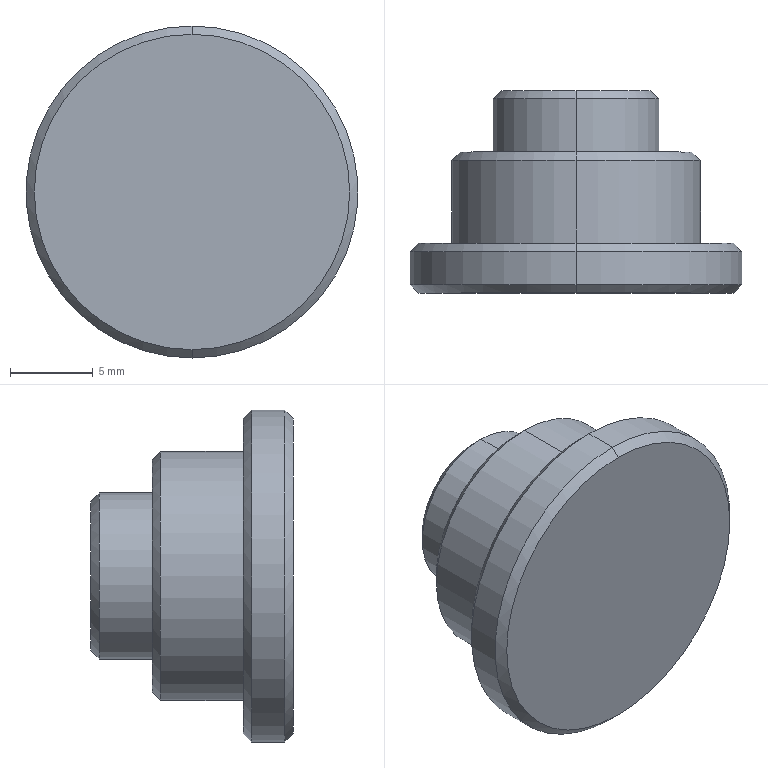Part | SolidWorks | features Chamfer 1, Revolution 1 | 1 solid | 18 faces | box 20 x 12.2 x 20 mm | volume 2180 mm3 | cone 8 | cylinder 6 | plane 4 | commonest cylinder face diameters 10 x2 15 x2 20 x2
STEP:
#1=CARTESIAN_POINT('',(136.663,-334.304,4.5));
#2=VERTEX_POINT('',#1);
#3=CARTESIAN_POINT('',(136.663,-334.304,-4.5));
#4=VERTEX_POINT('',#3);
#5=CARTESIAN_POINT('',(136.663,-334.304,0.));
#6=DIRECTION('',(0.,1.,0.));
#7=DIRECTION('',(0.,0.,-1.));
#8=AXIS2_PLACEMENT_3D('',#5,#6,#7);
#9=CIRCLE('',#8,4.5);
#10=EDGE_CURVE('',#2,#4,#9,.T.);
#11=ORIENTED_EDGE('',*,*,#10,.F.);
#12=CARTESIAN_POINT('',(136.663,-334.804,5.));
#13=VERTEX_POINT('',#12);
#14=CARTESIAN_POINT('',(136.663,-334.804,5.));
#15=DIRECTION('',(0.,-0.7071,0.7071));
#16=VECTOR('',#15,1000.);
#17=LINE('',#14,#16);
#18=EDGE_CURVE('',#2,#13,#17,.T.);
#19=ORIENTED_EDGE('',*,*,#18,.T.);
#20=CARTESIAN_POINT('',(136.663,-334.804,-5.));
#21=VERTEX_POINT('',#20);
#22=CARTESIAN_POINT('',(136.663,-334.804,0.));
#23=DIRECTION('',(0.,-1.,0.));
#24=DIRECTION('',(0.,0.,-1.));
#25=AXIS2_PLACEMENT_3D('',#22,#23,#24);
#26=CIRCLE('',#25,5.);
#27=EDGE_CURVE('',#21,#13,#26,.T.);
#28=ORIENTED_EDGE('',*,*,#27,.F.);
#29=CARTESIAN_POINT('',(136.663,-334.804,-5.));
#30=DIRECTION('',(0.,-0.7071,-0.7071));
#31=VECTOR('',#30,1000.);
#32=LINE('',#29,#31);
#33=EDGE_CURVE('',#4,#21,#32,.T.);
#34=ORIENTED_EDGE('',*,*,#33,.F.);
#35=EDGE_LOOP('',(#11,#19,#28,#34));
#36=FACE_OUTER_BOUND('',#35,.T.);
#37=CARTESIAN_POINT('',(136.663,-334.804,0.));
#38=DIRECTION('',(0.,-1.,0.));
#39=DIRECTION('',(0.,0.,-1.));
#40=AXIS2_PLACEMENT_3D('',#37,#38,#39);
#41=CONICAL_SURFACE('',#40,5.,0.7854);
#42=ADVANCED_FACE('',(#36),#41,.T.);
#43=CARTESIAN_POINT('',(136.663,-338.004,7.));
#44=VERTEX_POINT('',#43);
#45=CARTESIAN_POINT('',(136.663,-338.004,-7.));
#46=VERTEX_POINT('',#45);
#47=CARTESIAN_POINT('',(136.663,-338.004,0.));
#48=DIRECTION('',(0.,1.,0.));
#49=DIRECTION('',(0.,0.,-1.));
#50=AXIS2_PLACEMENT_3D('',#47,#48,#49);
#51=CIRCLE('',#50,7.);
#52=EDGE_CURVE('',#44,#46,#51,.T.);
#53=ORIENTED_EDGE('',*,*,#52,.F.);
#54=CARTESIAN_POINT('',(136.663,-338.504,7.5));
#55=VERTEX_POINT('',#54);
#56=CARTESIAN_POINT('',(136.663,-338.504,7.5));
#57=DIRECTION('',(0.,-0.7071,0.7071));
#58=VECTOR('',#57,1000.);
#59=LINE('',#56,#58);
#60=EDGE_CURVE('',#44,#55,#59,.T.);
#61=ORIENTED_EDGE('',*,*,#60,.T.);
#62=CARTESIAN_POINT('',(136.663,-338.504,-7.5));
#63=VERTEX_POINT('',#62);
#64=CARTESIAN_POINT('',(136.663,-338.504,0.));
#65=DIRECTION('',(0.,-1.,0.));
#66=DIRECTION('',(0.,0.,-1.));
#67=AXIS2_PLACEMENT_3D('',#64,#65,#66);
#68=CIRCLE('',#67,7.5);
#69=EDGE_CURVE('',#63,#55,#68,.T.);
#70=ORIENTED_EDGE('',*,*,#69,.F.);
#71=CARTESIAN_POINT('',(136.663,-338.504,-7.5));
#72=DIRECTION('',(0.,-0.7071,-0.7071));
#73=VECTOR('',#72,1000.);
#74=LINE('',#71,#73);
#75=EDGE_CURVE('',#46,#63,#74,.T.);
#76=ORIENTED_EDGE('',*,*,#75,.F.);
#77=EDGE_LOOP('',(#53,#61,#70,#76));
#78=FACE_OUTER_BOUND('',#77,.T.);
#79=CARTESIAN_POINT('',(136.663,-338.504,0.));
#80=DIRECTION('',(0.,-1.,0.));
#81=DIRECTION('',(0.,0.,-1.));
#82=AXIS2_PLACEMENT_3D('',#79,#80,#81);
#83=CONICAL_SURFACE('',#82,7.5,0.7854);
#84=ADVANCED_FACE('',(#78),#83,.T.);
#85=CARTESIAN_POINT('',(136.663,-343.504,9.5));
#86=VERTEX_POINT('',#85);
#87=CARTESIAN_POINT('',(136.663,-343.504,-9.5));
#88=VERTEX_POINT('',#87);
#89=CARTESIAN_POINT('',(136.663,-343.504,0.));
#90=DIRECTION('',(0.,1.,0.));
#91=DIRECTION('',(0.,0.,-1.));
#92=AXIS2_PLACEMENT_3D('',#89,#90,#91);
#93=CIRCLE('',#92,9.5);
#94=EDGE_CURVE('',#86,#88,#93,.T.);
#95=ORIENTED_EDGE('',*,*,#94,.F.);
#96=CARTESIAN_POINT('',(136.663,-344.004,10.));
#97=VERTEX_POINT('',#96);
#98=CARTESIAN_POINT('',(136.663,-344.004,10.));
#99=DIRECTION('',(0.,-0.7071,0.7071));
#100=VECTOR('',#99,1000.);
#101=LINE('',#98,#100);
#102=EDGE_CURVE('',#86,#97,#101,.T.);
#103=ORIENTED_EDGE('',*,*,#102,.T.);
#104=CARTESIAN_POINT('',(136.663,-344.004,-10.));
#105=VERTEX_POINT('',#104);
#106=CARTESIAN_POINT('',(136.663,-344.004,0.));
#107=DIRECTION('',(0.,-1.,0.));
#108=DIRECTION('',(0.,0.,-1.));
#109=AXIS2_PLACEMENT_3D('',#106,#107,#108);
#110=CIRCLE('',#109,10.);
#111=EDGE_CURVE('',#105,#97,#110,.T.);
#112=ORIENTED_EDGE('',*,*,#111,.F.);
#113=CARTESIAN_POINT('',(136.663,-344.004,-10.));
#114=DIRECTION('',(0.,-0.7071,-0.7071));
#115=VECTOR('',#114,1000.);
#116=LINE('',#113,#115);
#117=EDGE_CURVE('',#88,#105,#116,.T.);
#118=ORIENTED_EDGE('',*,*,#117,.F.);
#119=EDGE_LOOP('',(#95,#103,#112,#118));
#120=FACE_OUTER_BOUND('',#119,.T.);
#121=CARTESIAN_POINT('',(136.663,-344.004,0.));
#122=DIRECTION('',(0.,-1.,0.));
#123=DIRECTION('',(0.,0.,-1.));
#124=AXIS2_PLACEMENT_3D('',#121,#122,#123);
#125=CONICAL_SURFACE('',#124,10.,0.7854);
#126=ADVANCED_FACE('',(#120),#125,.T.);
#127=CARTESIAN_POINT('',(136.663,-346.504,-9.5));
#128=VERTEX_POINT('',#127);
#129=CARTESIAN_POINT('',(136.663,-346.504,9.5));
#130=VERTEX_POINT('',#129);
#131=CARTESIAN_POINT('',(136.663,-346.504,0.));
#132=DIRECTION('',(0.,-1.,0.));
#133=DIRECTION('',(0.,0.,1.));
#134=AXIS2_PLACEMENT_3D('',#131,#132,#133);
#135=CIRCLE('',#134,9.5);
#136=EDGE_CURVE('',#128,#130,#135,.T.);
#137=ORIENTED_EDGE('',*,*,#136,.F.);
#138=CARTESIAN_POINT('',(136.663,-346.004,-10.));
#139=VERTEX_POINT('',#138);
#140=CARTESIAN_POINT('',(136.663,-346.504,-9.5));
#141=DIRECTION('',(0.,0.7071,-0.7071));
#142=VECTOR('',#141,1000.);
#143=LINE('',#140,#142);
#144=EDGE_CURVE('',#128,#139,#143,.T.);
#145=ORIENTED_EDGE('',*,*,#144,.T.);
#146=CARTESIAN_POINT('',(136.663,-346.004,10.));
#147=VERTEX_POINT('',#146);
#148=CARTESIAN_POINT('',(136.663,-346.004,0.));
#149=DIRECTION('',(0.,1.,0.));
#150=DIRECTION('',(0.,0.,1.));
#151=AXIS2_PLACEMENT_3D('',#148,#149,#150);
#152=CIRCLE('',#151,10.);
#153=EDGE_CURVE('',#147,#139,#152,.T.);
#154=ORIENTED_EDGE('',*,*,#153,.F.);
#155=CARTESIAN_POINT('',(136.663,-346.504,9.5));
#156=DIRECTION('',(0.,0.7071,0.7071));
#157=VECTOR('',#156,1000.);
#158=LINE('',#155,#157);
#159=EDGE_CURVE('',#130,#147,#158,.T.);
#160=ORIENTED_EDGE('',*,*,#159,.F.);
#161=EDGE_LOOP('',(#137,#145,#154,#160));
#162=FACE_OUTER_BOUND('',#161,.T.);
#163=CARTESIAN_POINT('',(136.663,-346.504,0.));
#164=DIRECTION('',(0.,1.,0.));
#165=DIRECTION('',(0.,0.,1.));
#166=AXIS2_PLACEMENT_3D('',#163,#164,#165);
#167=CONICAL_SURFACE('',#166,9.5,0.7854);
#168=ADVANCED_FACE('',(#162),#167,.T.);
#169=ORIENTED_EDGE('',*,*,#111,.T.);
#170=CARTESIAN_POINT('',(136.663,-346.504,10.));
#171=DIRECTION('',(0.,-1.,0.));
#172=VECTOR('',#171,1000.);
#173=LINE('',#170,#172);
#174=EDGE_CURVE('',#97,#147,#173,.T.);
#175=ORIENTED_EDGE('',*,*,#174,.T.);
#176=ORIENTED_EDGE('',*,*,#153,.T.);
#177=CARTESIAN_POINT('',(136.663,-346.504,-10.));
#178=DIRECTION('',(0.,-1.,0.));
#179=VECTOR('',#178,1000.);
#180=LINE('',#177,#179);
#181=EDGE_CURVE('',#105,#139,#180,.T.);
#182=ORIENTED_EDGE('',*,*,#181,.F.);
#183=EDGE_LOOP('',(#169,#175,#176,#182));
#184=FACE_OUTER_BOUND('',#183,.T.);
#185=CARTESIAN_POINT('',(136.663,-346.504,0.));
#186=DIRECTION('',(0.,-1.,0.));
#187=DIRECTION('',(0.,0.,-1.));
#188=AXIS2_PLACEMENT_3D('',#185,#186,#187);
#189=CYLINDRICAL_SURFACE('',#188,10.);
#190=ADVANCED_FACE('',(#184),#189,.T.);
#191=ORIENTED_EDGE('',*,*,#69,.T.);
#192=CARTESIAN_POINT('',(136.663,-343.504,7.5));
#193=VERTEX_POINT('',#192);
#194=CARTESIAN_POINT('',(136.663,-346.504,7.5));
#195=DIRECTION('',(0.,-1.,0.));
#196=VECTOR('',#195,1000.);
#197=LINE('',#194,#196);
#198=EDGE_CURVE('',#55,#193,#197,.T.);
#199=ORIENTED_EDGE('',*,*,#198,.T.);
#200=CARTESIAN_POINT('',(136.663,-343.504,-7.5));
#201=VERTEX_POINT('',#200);
#202=CARTESIAN_POINT('',(136.663,-343.504,0.));
#203=DIRECTION('',(0.,-1.,0.));
#204=DIRECTION('',(0.,0.,-1.));
#205=AXIS2_PLACEMENT_3D('',#202,#203,#204);
#206=CIRCLE('',#205,7.5);
#207=EDGE_CURVE('',#201,#193,#206,.T.);
#208=ORIENTED_EDGE('',*,*,#207,.F.);
#209=CARTESIAN_POINT('',(136.663,-346.504,-7.5));
#210=DIRECTION('',(0.,-1.,0.));
#211=VECTOR('',#210,1000.);
#212=LINE('',#209,#211);
#213=EDGE_CURVE('',#63,#201,#212,.T.);
#214=ORIENTED_EDGE('',*,*,#213,.F.);
#215=EDGE_LOOP('',(#191,#199,#208,#214));
#216=FACE_OUTER_BOUND('',#215,.T.);
#217=CARTESIAN_POINT('',(136.663,-346.504,0.));
#218=DIRECTION('',(0.,-1.,0.));
#219=DIRECTION('',(0.,0.,-1.));
#220=AXIS2_PLACEMENT_3D('',#217,#218,#219);
#221=CYLINDRICAL_SURFACE('',#220,7.5);
#222=ADVANCED_FACE('',(#216),#221,.T.);
#223=ORIENTED_EDGE('',*,*,#27,.T.);
#224=CARTESIAN_POINT('',(136.663,-338.004,5.));
#225=VERTEX_POINT('',#224);
#226=CARTESIAN_POINT('',(136.663,-346.504,5.));
#227=DIRECTION('',(0.,-1.,0.));
#228=VECTOR('',#227,1000.);
#229=LINE('',#226,#228);
#230=EDGE_CURVE('',#13,#225,#229,.T.);
#231=ORIENTED_EDGE('',*,*,#230,.T.);
#232=CARTESIAN_POINT('',(136.663,-338.004,-5.));
#233=VERTEX_POINT('',#232);
#234=CARTESIAN_POINT('',(136.663,-338.004,0.));
#235=DIRECTION('',(0.,-1.,0.));
#236=DIRECTION('',(0.,0.,-1.));
#237=AXIS2_PLACEMENT_3D('',#234,#235,#236);
#238=CIRCLE('',#237,5.);
#239=EDGE_CURVE('',#233,#225,#238,.T.);
#240=ORIENTED_EDGE('',*,*,#239,.F.);
#241=CARTESIAN_POINT('',(136.663,-346.504,-5.));
#242=DIRECTION('',(0.,-1.,0.));
#243=VECTOR('',#242,1000.);
#244=LINE('',#241,#243);
#245=EDGE_CURVE('',#21,#233,#244,.T.);
#246=ORIENTED_EDGE('',*,*,#245,.F.);
#247=EDGE_LOOP('',(#223,#231,#240,#246));
#248=FACE_OUTER_BOUND('',#247,.T.);
#249=CARTESIAN_POINT('',(136.663,-346.504,0.));
#250=DIRECTION('',(0.,-1.,0.));
#251=DIRECTION('',(0.,0.,-1.));
#252=AXIS2_PLACEMENT_3D('',#249,#250,#251);
#253=CYLINDRICAL_SURFACE('',#252,5.);
#254=ADVANCED_FACE('',(#248),#253,.T.);
#255=CARTESIAN_POINT('',(136.663,-334.304,0.));
#256=DIRECTION('',(0.,1.,0.));
#257=DIRECTION('',(0.,0.,-1.));
#258=AXIS2_PLACEMENT_3D('',#255,#256,#257);
#259=CIRCLE('',#258,4.5);
#260=EDGE_CURVE('',#4,#2,#259,.T.);
#261=ORIENTED_EDGE('',*,*,#260,.T.);
#262=ORIENTED_EDGE('',*,*,#10,.T.);
#263=EDGE_LOOP('',(#261,#262));
#264=FACE_OUTER_BOUND('',#263,.T.);
#265=CARTESIAN_POINT('',(136.663,-334.304,0.));
#266=DIRECTION('',(0.,-1.,0.));
#267=DIRECTION('',(0.,0.,-1.));
#268=AXIS2_PLACEMENT_3D('',#265,#266,#267);
#269=PLANE('',#268);
#270=ADVANCED_FACE('',(#264),#269,.F.);
#271=ORIENTED_EDGE('',*,*,#230,.F.);
#272=CARTESIAN_POINT('',(136.663,-334.804,0.));
#273=DIRECTION('',(0.,-1.,0.));
#274=DIRECTION('',(0.,0.,-1.));
#275=AXIS2_PLACEMENT_3D('',#272,#273,#274);
#276=CIRCLE('',#275,5.);
#277=EDGE_CURVE('',#13,#21,#276,.T.);
#278=ORIENTED_EDGE('',*,*,#277,.T.);
#279=ORIENTED_EDGE('',*,*,#245,.T.);
#280=CARTESIAN_POINT('',(136.663,-338.004,0.));
#281=DIRECTION('',(0.,-1.,0.));
#282=DIRECTION('',(0.,0.,-1.));
#283=AXIS2_PLACEMENT_3D('',#280,#281,#282);
#284=CIRCLE('',#283,5.);
#285=EDGE_CURVE('',#225,#233,#284,.T.);
#286=ORIENTED_EDGE('',*,*,#285,.F.);
#287=EDGE_LOOP('',(#271,#278,#279,#286));
#288=FACE_OUTER_BOUND('',#287,.T.);
#289=CARTESIAN_POINT('',(136.663,-346.504,0.));
#290=DIRECTION('',(0.,-1.,0.));
#291=DIRECTION('',(0.,0.,-1.));
#292=AXIS2_PLACEMENT_3D('',#289,#290,#291);
#293=CYLINDRICAL_SURFACE('',#292,5.);
#294=ADVANCED_FACE('',(#288),#293,.T.);
#295=CARTESIAN_POINT('',(136.663,-338.004,0.));
#296=DIRECTION('',(0.,1.,0.));
#297=DIRECTION('',(0.,0.,-1.));
#298=AXIS2_PLACEMENT_3D('',#295,#296,#297);
#299=CIRCLE('',#298,7.);
#300=EDGE_CURVE('',#46,#44,#299,.T.);
#301=ORIENTED_EDGE('',*,*,#300,.T.);
#302=ORIENTED_EDGE('',*,*,#52,.T.);
#303=EDGE_LOOP('',(#301,#302));
#304=FACE_OUTER_BOUND('',#303,.T.);
#305=ORIENTED_EDGE('',*,*,#239,.T.);
#306=ORIENTED_EDGE('',*,*,#285,.T.);
#307=EDGE_LOOP('',(#305,#306));
#308=FACE_BOUND('',#307,.T.);
#309=CARTESIAN_POINT('',(131.663,-338.004,0.));
#310=DIRECTION('',(0.,-1.,0.));
#311=DIRECTION('',(0.,0.,-1.));
#312=AXIS2_PLACEMENT_3D('',#309,#310,#311);
#313=PLANE('',#312);
#314=ADVANCED_FACE('',(#304,#308),#313,.F.);
#315=ORIENTED_EDGE('',*,*,#198,.F.);
#316=CARTESIAN_POINT('',(136.663,-338.504,0.));
#317=DIRECTION('',(0.,-1.,0.));
#318=DIRECTION('',(0.,0.,-1.));
#319=AXIS2_PLACEMENT_3D('',#316,#317,#318);
#320=CIRCLE('',#319,7.5);
#321=EDGE_CURVE('',#55,#63,#320,.T.);
#322=ORIENTED_EDGE('',*,*,#321,.T.);
#323=ORIENTED_EDGE('',*,*,#213,.T.);
#324=CARTESIAN_POINT('',(136.663,-343.504,0.));
#325=DIRECTION('',(0.,-1.,0.));
#326=DIRECTION('',(0.,0.,-1.));
#327=AXIS2_PLACEMENT_3D('',#324,#325,#326);
#328=CIRCLE('',#327,7.5);
#329=EDGE_CURVE('',#193,#201,#328,.T.);
#330=ORIENTED_EDGE('',*,*,#329,.F.);
#331=EDGE_LOOP('',(#315,#322,#323,#330));
#332=FACE_OUTER_BOUND('',#331,.T.);
#333=CARTESIAN_POINT('',(136.663,-346.504,0.));
#334=DIRECTION('',(0.,-1.,0.));
#335=DIRECTION('',(0.,0.,-1.));
#336=AXIS2_PLACEMENT_3D('',#333,#334,#335);
#337=CYLINDRICAL_SURFACE('',#336,7.5);
#338=ADVANCED_FACE('',(#332),#337,.T.);
#339=CARTESIAN_POINT('',(136.663,-343.504,0.));
#340=DIRECTION('',(0.,1.,0.));
#341=DIRECTION('',(0.,0.,-1.));
#342=AXIS2_PLACEMENT_3D('',#339,#340,#341);
#343=CIRCLE('',#342,9.5);
#344=EDGE_CURVE('',#88,#86,#343,.T.);
#345=ORIENTED_EDGE('',*,*,#344,.T.);
#346=ORIENTED_EDGE('',*,*,#94,.T.);
#347=EDGE_LOOP('',(#345,#346));
#348=FACE_OUTER_BOUND('',#347,.T.);
#349=ORIENTED_EDGE('',*,*,#207,.T.);
#350=ORIENTED_EDGE('',*,*,#329,.T.);
#351=EDGE_LOOP('',(#349,#350));
#352=FACE_BOUND('',#351,.T.);
#353=CARTESIAN_POINT('',(129.163,-343.504,0.));
#354=DIRECTION('',(0.,-1.,0.));
#355=DIRECTION('',(0.,0.,-1.));
#356=AXIS2_PLACEMENT_3D('',#353,#354,#355);
#357=PLANE('',#356);
#358=ADVANCED_FACE('',(#348,#352),#357,.F.);
#359=ORIENTED_EDGE('',*,*,#174,.F.);
#360=CARTESIAN_POINT('',(136.663,-344.004,0.));
#361=DIRECTION('',(0.,-1.,0.));
#362=DIRECTION('',(0.,0.,-1.));
#363=AXIS2_PLACEMENT_3D('',#360,#361,#362);
#364=CIRCLE('',#363,10.);
#365=EDGE_CURVE('',#97,#105,#364,.T.);
#366=ORIENTED_EDGE('',*,*,#365,.T.);
#367=ORIENTED_EDGE('',*,*,#181,.T.);
#368=CARTESIAN_POINT('',(136.663,-346.004,0.));
#369=DIRECTION('',(0.,1.,0.));
#370=DIRECTION('',(0.,0.,1.));
#371=AXIS2_PLACEMENT_3D('',#368,#369,#370);
#372=CIRCLE('',#371,10.);
#373=EDGE_CURVE('',#139,#147,#372,.T.);
#374=ORIENTED_EDGE('',*,*,#373,.T.);
#375=EDGE_LOOP('',(#359,#366,#367,#374));
#376=FACE_OUTER_BOUND('',#375,.T.);
#377=CARTESIAN_POINT('',(136.663,-346.504,0.));
#378=DIRECTION('',(0.,-1.,0.));
#379=DIRECTION('',(0.,0.,-1.));
#380=AXIS2_PLACEMENT_3D('',#377,#378,#379);
#381=CYLINDRICAL_SURFACE('',#380,10.);
#382=ADVANCED_FACE('',(#376),#381,.T.);
#383=CARTESIAN_POINT('',(136.663,-346.504,0.));
#384=DIRECTION('',(0.,-1.,0.));
#385=DIRECTION('',(0.,0.,1.));
#386=AXIS2_PLACEMENT_3D('',#383,#384,#385);
#387=CIRCLE('',#386,9.5);
#388=EDGE_CURVE('',#130,#128,#387,.T.);
#389=ORIENTED_EDGE('',*,*,#388,.T.);
#390=ORIENTED_EDGE('',*,*,#136,.T.);
#391=EDGE_LOOP('',(#389,#390));
#392=FACE_OUTER_BOUND('',#391,.T.);
#393=CARTESIAN_POINT('',(126.663,-346.504,0.));
#394=DIRECTION('',(0.,1.,0.));
#395=DIRECTION('',(0.,0.,1.));
#396=AXIS2_PLACEMENT_3D('',#393,#394,#395);
#397=PLANE('',#396);
#398=ADVANCED_FACE('',(#392),#397,.F.);
#399=ORIENTED_EDGE('',*,*,#144,.F.);
#400=ORIENTED_EDGE('',*,*,#388,.F.);
#401=ORIENTED_EDGE('',*,*,#159,.T.);
#402=ORIENTED_EDGE('',*,*,#373,.F.);
#403=EDGE_LOOP('',(#399,#400,#401,#402));
#404=FACE_OUTER_BOUND('',#403,.T.);
#405=CARTESIAN_POINT('',(136.663,-346.504,0.));
#406=DIRECTION('',(0.,1.,0.));
#407=DIRECTION('',(0.,0.,1.));
#408=AXIS2_PLACEMENT_3D('',#405,#406,#407);
#409=CONICAL_SURFACE('',#408,9.5,0.7854);
#410=ADVANCED_FACE('',(#404),#409,.T.);
#411=ORIENTED_EDGE('',*,*,#102,.F.);
#412=ORIENTED_EDGE('',*,*,#344,.F.);
#413=ORIENTED_EDGE('',*,*,#117,.T.);
#414=ORIENTED_EDGE('',*,*,#365,.F.);
#415=EDGE_LOOP('',(#411,#412,#413,#414));
#416=FACE_OUTER_BOUND('',#415,.T.);
#417=CARTESIAN_POINT('',(136.663,-344.004,0.));
#418=DIRECTION('',(0.,-1.,0.));
#419=DIRECTION('',(0.,0.,-1.));
#420=AXIS2_PLACEMENT_3D('',#417,#418,#419);
#421=CONICAL_SURFACE('',#420,10.,0.7854);
#422=ADVANCED_FACE('',(#416),#421,.T.);
#423=ORIENTED_EDGE('',*,*,#60,.F.);
#424=ORIENTED_EDGE('',*,*,#300,.F.);
#425=ORIENTED_EDGE('',*,*,#75,.T.);
#426=ORIENTED_EDGE('',*,*,#321,.F.);
#427=EDGE_LOOP('',(#423,#424,#425,#426));
#428=FACE_OUTER_BOUND('',#427,.T.);
#429=CARTESIAN_POINT('',(136.663,-338.504,0.));
#430=DIRECTION('',(0.,-1.,0.));
#431=DIRECTION('',(0.,0.,-1.));
#432=AXIS2_PLACEMENT_3D('',#429,#430,#431);
#433=CONICAL_SURFACE('',#432,7.5,0.7854);
#434=ADVANCED_FACE('',(#428),#433,.T.);
#435=ORIENTED_EDGE('',*,*,#18,.F.);
#436=ORIENTED_EDGE('',*,*,#260,.F.);
#437=ORIENTED_EDGE('',*,*,#33,.T.);
#438=ORIENTED_EDGE('',*,*,#277,.F.);
#439=EDGE_LOOP('',(#435,#436,#437,#438));
#440=FACE_OUTER_BOUND('',#439,.T.);
#441=CARTESIAN_POINT('',(136.663,-334.804,0.));
#442=DIRECTION('',(0.,-1.,0.));
#443=DIRECTION('',(0.,0.,-1.));
#444=AXIS2_PLACEMENT_3D('',#441,#442,#443);
#445=CONICAL_SURFACE('',#444,5.,0.7854);
#446=ADVANCED_FACE('',(#440),#445,.T.);
#447=CLOSED_SHELL('',(#42,#84,#126,#168,#190,#222,#254,#270,#294,#314,#338,#358,#382,#398,#410,#422,#434,#446));
#448=MANIFOLD_SOLID_BREP('',#447);
#449=CARTESIAN_POINT('',(0.,0.,0.));
#450=DIRECTION('',(0.,0.,1.));
#451=DIRECTION('',(1.,0.,0.));
#452=AXIS2_PLACEMENT_3D('',#449,#450,#451);
#453=(LENGTH_UNIT()NAMED_UNIT(*)SI_UNIT(.MILLI.,.METRE.));
#454=UNCERTAINTY_MEASURE_WITH_UNIT(LENGTH_MEASURE(0.00001),#453,'','');
#455=(NAMED_UNIT(*)PLANE_ANGLE_UNIT()SI_UNIT($,.RADIAN.));
#456=(NAMED_UNIT(*)SI_UNIT($,.STERADIAN.)SOLID_ANGLE_UNIT());
#457=(GEOMETRIC_REPRESENTATION_CONTEXT(3)GLOBAL_UNCERTAINTY_ASSIGNED_CONTEXT((#454))GLOBAL_UNIT_ASSIGNED_CONTEXT((#453,#455,#456))REPRESENTATION_CONTEXT('',''));
#458=ADVANCED_BREP_SHAPE_REPRESENTATION('',(#448,#452),#457);